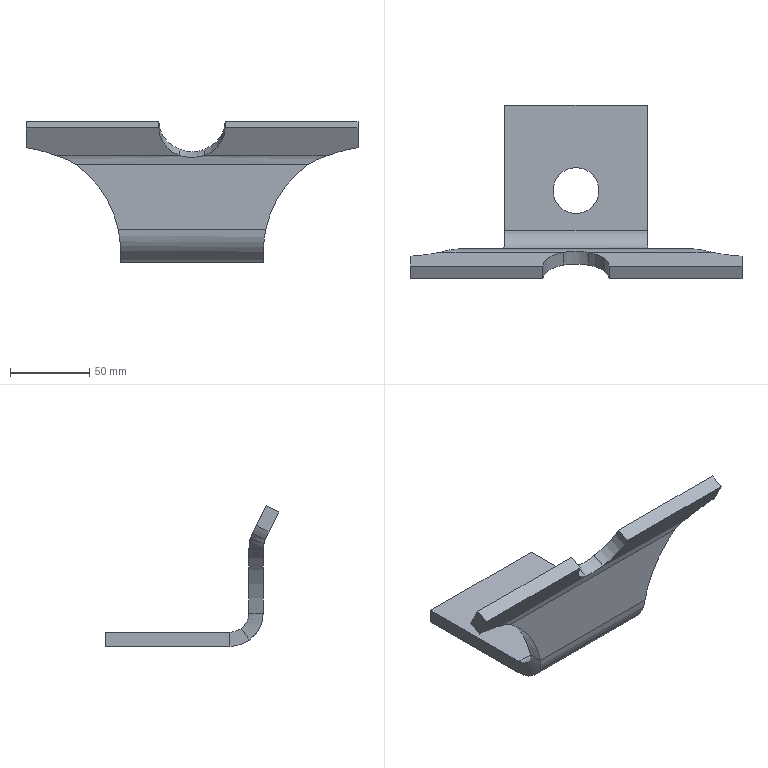Part | SolidWorks | features SM3dBend 2, FlatPattern 1, SMBaseFlange 1, SheetMetal 1, UnFold 1 | 1 solid | 34 faces | box 210 x 110.002 x 89.027 mm | volume 161533 mm3 | plane 17 | cylinder 12 | spline 5 | commonest cylinder face diameters 42 x4 140 x4 24 x2 29 x2
STEP:
#1=CARTESIAN_POINT('',(-14.5,118.35,9.));
#2=VERTEX_POINT('',#1);
#3=CARTESIAN_POINT('',(14.5,118.35,9.));
#4=VERTEX_POINT('',#3);
#5=CARTESIAN_POINT('',(0.,118.35,9.));
#6=DIRECTION('',(0.,0.,1.));
#7=DIRECTION('',(1.,0.,0.));
#8=AXIS2_PLACEMENT_3D('',#5,#6,#7);
#9=CIRCLE('',#8,14.5);
#10=EDGE_CURVE('',#2,#4,#9,.T.);
#11=ORIENTED_EDGE('',*,*,#10,.T.);
#12=CARTESIAN_POINT('',(14.5,118.35,0.));
#13=VERTEX_POINT('',#12);
#14=CARTESIAN_POINT('',(14.5,118.35,9.));
#15=DIRECTION('',(0.,0.,-1.));
#16=VECTOR('',#15,1000.);
#17=LINE('',#14,#16);
#18=EDGE_CURVE('',#4,#13,#17,.T.);
#19=ORIENTED_EDGE('',*,*,#18,.T.);
#20=CARTESIAN_POINT('',(-14.5,118.35,0.));
#21=VERTEX_POINT('',#20);
#22=CARTESIAN_POINT('',(0.,118.35,0.));
#23=DIRECTION('',(0.,0.,1.));
#24=DIRECTION('',(1.,0.,0.));
#25=AXIS2_PLACEMENT_3D('',#22,#23,#24);
#26=CIRCLE('',#25,14.5);
#27=EDGE_CURVE('',#21,#13,#26,.T.);
#28=ORIENTED_EDGE('',*,*,#27,.F.);
#29=CARTESIAN_POINT('',(-14.5,118.35,9.));
#30=DIRECTION('',(0.,0.,-1.));
#31=VECTOR('',#30,1000.);
#32=LINE('',#29,#31);
#33=EDGE_CURVE('',#2,#21,#32,.T.);
#34=ORIENTED_EDGE('',*,*,#33,.F.);
#35=EDGE_LOOP('',(#11,#19,#28,#34));
#36=FACE_OUTER_BOUND('',#35,.T.);
#37=CARTESIAN_POINT('',(0.,118.35,9.));
#38=DIRECTION('',(0.,0.,-1.));
#39=DIRECTION('',(-1.,0.,0.));
#40=AXIS2_PLACEMENT_3D('',#37,#38,#39);
#41=CYLINDRICAL_SURFACE('',#40,14.5);
#42=ADVANCED_FACE('',(#36),#41,.F.);
#43=CARTESIAN_POINT('',(-46.658,81.35,21.));
#44=VERTEX_POINT('',#43);
#45=CARTESIAN_POINT('',(-73.419,81.35,62.169));
#46=VERTEX_POINT('',#45);
#47=CARTESIAN_POINT('',(-115.,81.35,5.857));
#48=DIRECTION('',(0.,-1.,0.));
#49=DIRECTION('',(-1.,0.,0.));
#50=AXIS2_PLACEMENT_3D('',#47,#48,#49);
#51=CIRCLE('',#50,70.);
#52=EDGE_CURVE('',#44,#46,#51,.T.);
#53=ORIENTED_EDGE('',*,*,#52,.T.);
#54=CARTESIAN_POINT('',(73.419,81.35,62.169));
#55=VERTEX_POINT('',#54);
#56=CARTESIAN_POINT('',(115.,81.35,62.169));
#57=DIRECTION('',(1.,0.,0.));
#58=VECTOR('',#57,1000.);
#59=LINE('',#56,#58);
#60=EDGE_CURVE('',#46,#55,#59,.T.);
#61=ORIENTED_EDGE('',*,*,#60,.T.);
#62=CARTESIAN_POINT('',(46.658,81.35,21.));
#63=VERTEX_POINT('',#62);
#64=CARTESIAN_POINT('',(115.,81.35,5.857));
#65=DIRECTION('',(0.,-1.,0.));
#66=DIRECTION('',(1.,0.,0.));
#67=AXIS2_PLACEMENT_3D('',#64,#65,#66);
#68=CIRCLE('',#67,70.);
#69=EDGE_CURVE('',#55,#63,#68,.T.);
#70=ORIENTED_EDGE('',*,*,#69,.T.);
#71=CARTESIAN_POINT('',(115.,81.35,21.));
#72=DIRECTION('',(1.,0.,0.));
#73=VECTOR('',#72,1000.);
#74=LINE('',#71,#73);
#75=EDGE_CURVE('',#44,#63,#74,.T.);
#76=ORIENTED_EDGE('',*,*,#75,.F.);
#77=EDGE_LOOP('',(#53,#61,#70,#76));
#78=FACE_OUTER_BOUND('',#77,.T.);
#79=CARTESIAN_POINT('',(115.,81.35,5.857));
#80=DIRECTION('',(0.,1.,0.));
#81=DIRECTION('',(1.,0.,0.));
#82=AXIS2_PLACEMENT_3D('',#79,#80,#81);
#83=PLANE('',#82);
#84=ADVANCED_FACE('',(#78),#83,.T.);
#85=CARTESIAN_POINT('',(-73.419,72.35,62.169));
#86=VERTEX_POINT('',#85);
#87=CARTESIAN_POINT('',(-73.419,81.35,62.169));
#88=CARTESIAN_POINT('',(-73.419,72.35,62.169));
#89=B_SPLINE_CURVE_WITH_KNOTS('',1,(#87,#88),.UNSPECIFIED.,.F.,.F.,(2,2),(0.,1.),.UNSPECIFIED.);
#90=EDGE_CURVE('',#46,#86,#89,.T.);
#91=ORIENTED_EDGE('',*,*,#90,.F.);
#92=ORIENTED_EDGE('',*,*,#52,.F.);
#93=CARTESIAN_POINT('',(-46.658,72.35,21.));
#94=VERTEX_POINT('',#93);
#95=CARTESIAN_POINT('',(-46.658,81.35,21.));
#96=CARTESIAN_POINT('',(-46.658,78.35,21.));
#97=CARTESIAN_POINT('',(-46.658,75.35,21.));
#98=CARTESIAN_POINT('',(-46.658,72.35,21.));
#99=B_SPLINE_CURVE_WITH_KNOTS('',3,(#95,#96,#97,#98),.UNSPECIFIED.,.F.,.F.,(4,4),(0.,1.),.UNSPECIFIED.);
#100=EDGE_CURVE('',#44,#94,#99,.T.);
#101=ORIENTED_EDGE('',*,*,#100,.T.);
#102=CARTESIAN_POINT('',(-115.,72.35,5.857));
#103=DIRECTION('',(0.,-1.,0.));
#104=DIRECTION('',(-1.,0.,0.));
#105=AXIS2_PLACEMENT_3D('',#102,#103,#104);
#106=CIRCLE('',#105,70.);
#107=EDGE_CURVE('',#94,#86,#106,.T.);
#108=ORIENTED_EDGE('',*,*,#107,.T.);
#109=EDGE_LOOP('',(#91,#92,#101,#108));
#110=FACE_OUTER_BOUND('',#109,.T.);
#111=CARTESIAN_POINT('',(-115.,81.35,5.857));
#112=DIRECTION('',(0.,-1.,0.));
#113=DIRECTION('',(-1.,0.,0.));
#114=AXIS2_PLACEMENT_3D('',#111,#112,#113);
#115=CYLINDRICAL_SURFACE('',#114,70.);
#116=ADVANCED_FACE('',(#110),#115,.F.);
#117=CARTESIAN_POINT('',(73.419,72.35,62.169));
#118=VERTEX_POINT('',#117);
#119=CARTESIAN_POINT('',(73.419,72.35,62.169));
#120=CARTESIAN_POINT('',(73.419,81.35,62.169));
#121=B_SPLINE_CURVE_WITH_KNOTS('',1,(#119,#120),.UNSPECIFIED.,.F.,.F.,(2,2),(0.,1.),.UNSPECIFIED.);
#122=EDGE_CURVE('',#118,#55,#121,.T.);
#123=ORIENTED_EDGE('',*,*,#122,.F.);
#124=CARTESIAN_POINT('',(46.658,72.35,21.));
#125=VERTEX_POINT('',#124);
#126=CARTESIAN_POINT('',(115.,72.35,5.857));
#127=DIRECTION('',(0.,-1.,0.));
#128=DIRECTION('',(1.,0.,0.));
#129=AXIS2_PLACEMENT_3D('',#126,#127,#128);
#130=CIRCLE('',#129,70.);
#131=EDGE_CURVE('',#118,#125,#130,.T.);
#132=ORIENTED_EDGE('',*,*,#131,.T.);
#133=CARTESIAN_POINT('',(46.658,72.35,21.));
#134=CARTESIAN_POINT('',(46.658,75.35,21.));
#135=CARTESIAN_POINT('',(46.658,78.35,21.));
#136=CARTESIAN_POINT('',(46.658,81.35,21.));
#137=B_SPLINE_CURVE_WITH_KNOTS('',3,(#133,#134,#135,#136),.UNSPECIFIED.,.F.,.F.,(4,4),(0.,1.),.UNSPECIFIED.);
#138=EDGE_CURVE('',#125,#63,#137,.T.);
#139=ORIENTED_EDGE('',*,*,#138,.T.);
#140=ORIENTED_EDGE('',*,*,#69,.F.);
#141=EDGE_LOOP('',(#123,#132,#139,#140));
#142=FACE_OUTER_BOUND('',#141,.T.);
#143=CARTESIAN_POINT('',(115.,81.35,5.857));
#144=DIRECTION('',(0.,-1.,0.));
#145=DIRECTION('',(-1.,0.,0.));
#146=AXIS2_PLACEMENT_3D('',#143,#144,#145);
#147=CYLINDRICAL_SURFACE('',#146,70.);
#148=ADVANCED_FACE('',(#142),#147,.F.);
#149=CARTESIAN_POINT('',(115.,72.35,62.169));
#150=DIRECTION('',(1.,0.,0.));
#151=VECTOR('',#150,1000.);
#152=LINE('',#149,#151);
#153=EDGE_CURVE('',#86,#118,#152,.T.);
#154=ORIENTED_EDGE('',*,*,#153,.F.);
#155=ORIENTED_EDGE('',*,*,#107,.F.);
#156=CARTESIAN_POINT('',(115.,72.35,21.));
#157=DIRECTION('',(1.,0.,0.));
#158=VECTOR('',#157,1000.);
#159=LINE('',#156,#158);
#160=EDGE_CURVE('',#94,#125,#159,.T.);
#161=ORIENTED_EDGE('',*,*,#160,.T.);
#162=ORIENTED_EDGE('',*,*,#131,.F.);
#163=EDGE_LOOP('',(#154,#155,#161,#162));
#164=FACE_OUTER_BOUND('',#163,.T.);
#165=CARTESIAN_POINT('',(115.,72.35,5.857));
#166=DIRECTION('',(0.,1.,0.));
#167=DIRECTION('',(1.,0.,0.));
#168=AXIS2_PLACEMENT_3D('',#165,#166,#167);
#169=PLANE('',#168);
#170=ADVANCED_FACE('',(#164),#169,.F.);
#171=CARTESIAN_POINT('',(45.,172.35,0.));
#172=VERTEX_POINT('',#171);
#173=CARTESIAN_POINT('',(-45.,172.35,0.));
#174=VERTEX_POINT('',#173);
#175=CARTESIAN_POINT('',(45.,172.35,0.));
#176=DIRECTION('',(-1.,0.,0.));
#177=VECTOR('',#176,1000.);
#178=LINE('',#175,#177);
#179=EDGE_CURVE('',#172,#174,#178,.T.);
#180=ORIENTED_EDGE('',*,*,#179,.T.);
#181=CARTESIAN_POINT('',(-45.,172.35,9.));
#182=VERTEX_POINT('',#181);
#183=CARTESIAN_POINT('',(-45.,172.35,9.));
#184=DIRECTION('',(0.,0.,-1.));
#185=VECTOR('',#184,1000.);
#186=LINE('',#183,#185);
#187=EDGE_CURVE('',#182,#174,#186,.T.);
#188=ORIENTED_EDGE('',*,*,#187,.F.);
#189=CARTESIAN_POINT('',(45.,172.35,9.));
#190=VERTEX_POINT('',#189);
#191=CARTESIAN_POINT('',(45.,172.35,9.));
#192=DIRECTION('',(-1.,0.,0.));
#193=VECTOR('',#192,1000.);
#194=LINE('',#191,#193);
#195=EDGE_CURVE('',#190,#182,#194,.T.);
#196=ORIENTED_EDGE('',*,*,#195,.F.);
#197=CARTESIAN_POINT('',(45.,172.35,9.));
#198=DIRECTION('',(0.,0.,-1.));
#199=VECTOR('',#198,1000.);
#200=LINE('',#197,#199);
#201=EDGE_CURVE('',#190,#172,#200,.T.);
#202=ORIENTED_EDGE('',*,*,#201,.T.);
#203=EDGE_LOOP('',(#180,#188,#196,#202));
#204=FACE_OUTER_BOUND('',#203,.T.);
#205=CARTESIAN_POINT('',(45.,172.35,9.));
#206=DIRECTION('',(0.,-1.,0.));
#207=DIRECTION('',(0.,0.,-1.));
#208=AXIS2_PLACEMENT_3D('',#205,#206,#207);
#209=PLANE('',#208);
#210=ADVANCED_FACE('',(#204),#209,.F.);
#211=ORIENTED_EDGE('',*,*,#18,.F.);
#212=CARTESIAN_POINT('',(0.,118.35,9.));
#213=DIRECTION('',(0.,0.,1.));
#214=DIRECTION('',(1.,0.,0.));
#215=AXIS2_PLACEMENT_3D('',#212,#213,#214);
#216=CIRCLE('',#215,14.5);
#217=EDGE_CURVE('',#4,#2,#216,.T.);
#218=ORIENTED_EDGE('',*,*,#217,.T.);
#219=ORIENTED_EDGE('',*,*,#33,.T.);
#220=CARTESIAN_POINT('',(0.,118.35,0.));
#221=DIRECTION('',(0.,0.,1.));
#222=DIRECTION('',(1.,0.,0.));
#223=AXIS2_PLACEMENT_3D('',#220,#221,#222);
#224=CIRCLE('',#223,14.5);
#225=EDGE_CURVE('',#13,#21,#224,.T.);
#226=ORIENTED_EDGE('',*,*,#225,.F.);
#227=EDGE_LOOP('',(#211,#218,#219,#226));
#228=FACE_OUTER_BOUND('',#227,.T.);
#229=CARTESIAN_POINT('',(0.,118.35,9.));
#230=DIRECTION('',(0.,0.,-1.));
#231=DIRECTION('',(-1.,0.,0.));
#232=AXIS2_PLACEMENT_3D('',#229,#230,#231);
#233=CYLINDRICAL_SURFACE('',#232,14.5);
#234=ADVANCED_FACE('',(#228),#233,.F.);
#235=ORIENTED_EDGE('',*,*,#10,.F.);
#236=ORIENTED_EDGE('',*,*,#217,.F.);
#237=EDGE_LOOP('',(#235,#236));
#238=FACE_BOUND('',#237,.T.);
#239=CARTESIAN_POINT('',(-45.,93.35,9.));
#240=VERTEX_POINT('',#239);
#241=CARTESIAN_POINT('',(-45.,83.282,9.));
#242=DIRECTION('',(0.,-1.,0.));
#243=VECTOR('',#242,1000.);
#244=LINE('',#241,#243);
#245=EDGE_CURVE('',#182,#240,#244,.T.);
#246=ORIENTED_EDGE('',*,*,#245,.T.);
#247=CARTESIAN_POINT('',(45.,93.35,9.));
#248=VERTEX_POINT('',#247);
#249=CARTESIAN_POINT('',(115.,93.35,9.));
#250=DIRECTION('',(1.,0.,0.));
#251=VECTOR('',#250,1000.);
#252=LINE('',#249,#251);
#253=EDGE_CURVE('',#240,#248,#252,.T.);
#254=ORIENTED_EDGE('',*,*,#253,.T.);
#255=CARTESIAN_POINT('',(45.,83.282,9.));
#256=DIRECTION('',(0.,1.,0.));
#257=VECTOR('',#256,1000.);
#258=LINE('',#255,#257);
#259=EDGE_CURVE('',#248,#190,#258,.T.);
#260=ORIENTED_EDGE('',*,*,#259,.T.);
#261=ORIENTED_EDGE('',*,*,#195,.T.);
#262=EDGE_LOOP('',(#246,#254,#260,#261));
#263=FACE_OUTER_BOUND('',#262,.T.);
#264=CARTESIAN_POINT('',(115.,83.282,9.));
#265=DIRECTION('',(0.,0.,1.));
#266=DIRECTION('',(1.,0.,0.));
#267=AXIS2_PLACEMENT_3D('',#264,#265,#266);
#268=PLANE('',#267);
#269=ADVANCED_FACE('',(#238,#263),#268,.T.);
#270=CARTESIAN_POINT('',(45.,93.35,0.));
#271=VERTEX_POINT('',#270);
#272=CARTESIAN_POINT('',(45.,93.35,9.));
#273=DIRECTION('',(0.,0.,1.));
#274=VECTOR('',#273,1000.);
#275=LINE('',#272,#274);
#276=EDGE_CURVE('',#271,#248,#275,.T.);
#277=ORIENTED_EDGE('',*,*,#276,.F.);
#278=CARTESIAN_POINT('',(45.,83.282,0.));
#279=DIRECTION('',(0.,1.,0.));
#280=VECTOR('',#279,1000.);
#281=LINE('',#278,#280);
#282=EDGE_CURVE('',#271,#172,#281,.T.);
#283=ORIENTED_EDGE('',*,*,#282,.T.);
#284=ORIENTED_EDGE('',*,*,#201,.F.);
#285=ORIENTED_EDGE('',*,*,#259,.F.);
#286=EDGE_LOOP('',(#277,#283,#284,#285));
#287=FACE_OUTER_BOUND('',#286,.T.);
#288=CARTESIAN_POINT('',(45.,83.282,9.));
#289=DIRECTION('',(-1.,0.,0.));
#290=DIRECTION('',(0.,0.,1.));
#291=AXIS2_PLACEMENT_3D('',#288,#289,#290);
#292=PLANE('',#291);
#293=ADVANCED_FACE('',(#287),#292,.F.);
#294=CARTESIAN_POINT('',(-45.,93.35,0.));
#295=VERTEX_POINT('',#294);
#296=CARTESIAN_POINT('',(115.,93.35,0.));
#297=DIRECTION('',(1.,0.,0.));
#298=VECTOR('',#297,1000.);
#299=LINE('',#296,#298);
#300=EDGE_CURVE('',#295,#271,#299,.T.);
#301=ORIENTED_EDGE('',*,*,#300,.F.);
#302=CARTESIAN_POINT('',(-45.,83.282,0.));
#303=DIRECTION('',(0.,-1.,0.));
#304=VECTOR('',#303,1000.);
#305=LINE('',#302,#304);
#306=EDGE_CURVE('',#174,#295,#305,.T.);
#307=ORIENTED_EDGE('',*,*,#306,.F.);
#308=ORIENTED_EDGE('',*,*,#179,.F.);
#309=ORIENTED_EDGE('',*,*,#282,.F.);
#310=EDGE_LOOP('',(#301,#307,#308,#309));
#311=FACE_OUTER_BOUND('',#310,.T.);
#312=ORIENTED_EDGE('',*,*,#27,.T.);
#313=ORIENTED_EDGE('',*,*,#225,.T.);
#314=EDGE_LOOP('',(#312,#313));
#315=FACE_BOUND('',#314,.T.);
#316=CARTESIAN_POINT('',(115.,83.282,0.));
#317=DIRECTION('',(0.,0.,1.));
#318=DIRECTION('',(1.,0.,0.));
#319=AXIS2_PLACEMENT_3D('',#316,#317,#318);
#320=PLANE('',#319);
#321=ADVANCED_FACE('',(#311,#315),#320,.F.);
#322=CARTESIAN_POINT('',(-45.,93.35,9.));
#323=DIRECTION('',(0.,0.,-1.));
#324=VECTOR('',#323,1000.);
#325=LINE('',#322,#324);
#326=EDGE_CURVE('',#240,#295,#325,.T.);
#327=ORIENTED_EDGE('',*,*,#326,.F.);
#328=ORIENTED_EDGE('',*,*,#245,.F.);
#329=ORIENTED_EDGE('',*,*,#187,.T.);
#330=ORIENTED_EDGE('',*,*,#306,.T.);
#331=EDGE_LOOP('',(#327,#328,#329,#330));
#332=FACE_OUTER_BOUND('',#331,.T.);
#333=CARTESIAN_POINT('',(-45.,83.282,9.));
#334=DIRECTION('',(1.,0.,0.));
#335=DIRECTION('',(0.,0.,-1.));
#336=AXIS2_PLACEMENT_3D('',#333,#334,#335);
#337=PLANE('',#336);
#338=ADVANCED_FACE('',(#332),#337,.F.);
#339=CARTESIAN_POINT('',(-45.,81.024,3.998));
#340=VERTEX_POINT('',#339);
#341=CARTESIAN_POINT('',(-45.,86.307,11.285));
#342=VERTEX_POINT('',#341);
#343=CARTESIAN_POINT('',(-45.,81.024,3.998));
#344=CARTESIAN_POINT('',(-45.,82.785,6.427));
#345=CARTESIAN_POINT('',(-45.,84.546,8.856));
#346=CARTESIAN_POINT('',(-45.,86.307,11.285));
#347=B_SPLINE_CURVE_WITH_KNOTS('',3,(#343,#344,#345,#346),.UNSPECIFIED.,.F.,.F.,(4,4),(0.,1.),.UNSPECIFIED.);
#348=EDGE_CURVE('',#340,#342,#347,.T.);
#349=ORIENTED_EDGE('',*,*,#348,.F.);
#350=CARTESIAN_POINT('',(-45.,81.024,3.998));
#351=CARTESIAN_POINT('',(-45.037,79.286,5.258));
#352=CARTESIAN_POINT('',(-45.09,77.943,6.633));
#353=CARTESIAN_POINT('',(-45.193,76.386,8.593));
#354=CARTESIAN_POINT('',(-45.231,75.943,9.231));
#355=CARTESIAN_POINT('',(-45.294,75.372,10.141));
#356=CARTESIAN_POINT('',(-45.316,75.197,10.436));
#357=CARTESIAN_POINT('',(-45.362,74.876,11.009));
#358=CARTESIAN_POINT('',(-45.385,74.733,11.278));
#359=CARTESIAN_POINT('',(-45.513,74.041,12.652));
#360=CARTESIAN_POINT('',(-45.669,73.49,13.982));
#361=CARTESIAN_POINT('',(-46.084,72.644,17.137));
#362=CARTESIAN_POINT('',(-46.344,72.35,18.962));
#363=CARTESIAN_POINT('',(-46.658,72.35,21.));
#364=B_SPLINE_CURVE_WITH_KNOTS('',3,(#350,#351,#352,#353,#354,#355,#356,#357,#358,#359,#360,#361,#362,#363),.UNSPECIFIED.,.F.,.F.,(4,2,2,2,2,2,4),(0.,0.25,0.375,0.4375,0.5,0.75,1.),.UNSPECIFIED.);
#365=EDGE_CURVE('',#340,#94,#364,.T.);
#366=ORIENTED_EDGE('',*,*,#365,.T.);
#367=ORIENTED_EDGE('',*,*,#100,.F.);
#368=CARTESIAN_POINT('',(-45.,86.307,11.285));
#369=CARTESIAN_POINT('',(-45.037,85.315,12.003));
#370=CARTESIAN_POINT('',(-45.09,84.546,12.79));
#371=CARTESIAN_POINT('',(-45.193,83.656,13.91));
#372=CARTESIAN_POINT('',(-45.231,83.403,14.275));
#373=CARTESIAN_POINT('',(-45.294,83.077,14.795));
#374=CARTESIAN_POINT('',(-45.316,82.977,14.964));
#375=CARTESIAN_POINT('',(-45.35,82.839,15.209));
#376=CARTESIAN_POINT('',(-45.368,82.773,15.33));
#377=CARTESIAN_POINT('',(-45.386,82.712,15.447));
#378=CARTESIAN_POINT('',(-45.398,82.672,15.525));
#379=CARTESIAN_POINT('',(-45.404,82.653,15.562));
#380=CARTESIAN_POINT('',(-45.513,82.317,16.23));
#381=CARTESIAN_POINT('',(-45.669,82.002,16.99));
#382=CARTESIAN_POINT('',(-46.084,81.518,18.792));
#383=CARTESIAN_POINT('',(-46.345,81.35,19.837));
#384=CARTESIAN_POINT('',(-46.658,81.35,21.));
#385=B_SPLINE_CURVE_WITH_KNOTS('',3,(#368,#369,#370,#371,#372,#373,#374,#375,#376,#377,#378,#379,#380,#381,#382,#383,#384),.UNSPECIFIED.,.F.,.F.,(4,2,2,2,1,2,2,2,4),(0.,0.25,0.375,0.4375,0.4688,0.4844,0.5,0.75,1.),.UNSPECIFIED.);
#386=EDGE_CURVE('',#342,#44,#385,.T.);
#387=ORIENTED_EDGE('',*,*,#386,.F.);
#388=EDGE_LOOP('',(#349,#366,#367,#387));
#389=FACE_OUTER_BOUND('',#388,.T.);
#390=CARTESIAN_POINT('',(-45.,81.024,3.998));
#391=CARTESIAN_POINT('',(-45.037,79.286,5.258));
#392=CARTESIAN_POINT('',(-45.09,77.943,6.633));
#393=CARTESIAN_POINT('',(-45.193,76.386,8.593));
#394=CARTESIAN_POINT('',(-45.231,75.943,9.231));
#395=CARTESIAN_POINT('',(-45.294,75.372,10.141));
#396=CARTESIAN_POINT('',(-45.316,75.197,10.436));
#397=CARTESIAN_POINT('',(-45.362,74.876,11.009));
#398=CARTESIAN_POINT('',(-45.385,74.733,11.278));
#399=CARTESIAN_POINT('',(-45.513,74.041,12.652));
#400=CARTESIAN_POINT('',(-45.669,73.49,13.982));
#401=CARTESIAN_POINT('',(-46.084,72.644,17.137));
#402=CARTESIAN_POINT('',(-46.344,72.35,18.962));
#403=CARTESIAN_POINT('',(-46.658,72.35,21.));
#404=CARTESIAN_POINT('',(-45.,86.307,11.285));
#405=CARTESIAN_POINT('',(-45.037,85.314,12.004));
#406=CARTESIAN_POINT('',(-45.09,84.546,12.79));
#407=CARTESIAN_POINT('',(-45.193,83.656,13.91));
#408=CARTESIAN_POINT('',(-45.231,83.403,14.275));
#409=CARTESIAN_POINT('',(-45.294,83.077,14.795));
#410=CARTESIAN_POINT('',(-45.316,82.977,14.964));
#411=CARTESIAN_POINT('',(-45.362,82.793,15.291));
#412=CARTESIAN_POINT('',(-45.385,82.712,15.445));
#413=CARTESIAN_POINT('',(-45.513,82.317,16.23));
#414=CARTESIAN_POINT('',(-45.669,82.002,16.99));
#415=CARTESIAN_POINT('',(-46.084,81.518,18.792));
#416=CARTESIAN_POINT('',(-46.344,81.35,19.835));
#417=CARTESIAN_POINT('',(-46.658,81.35,21.));
#418=B_SPLINE_SURFACE_WITH_KNOTS('',1,3,((#390,#391,#392,#393,#394,#395,#396,#397,#398,#399,#400,#401,#402,#403),(#404,#405,#406,#407,#408,#409,#410,#411,#412,#413,#414,#415,#416,#417)),.UNSPECIFIED.,.F.,.F.,.F.,(2,2),(4,2,2,2,2,2,4),(0.,1.),(0.,0.25,0.375,0.4375,0.5,0.75,1.),.UNSPECIFIED.);
#419=ADVANCED_FACE('',(#389),#418,.F.);
#420=ORIENTED_EDGE('',*,*,#138,.F.);
#421=CARTESIAN_POINT('',(45.,81.024,3.998));
#422=VERTEX_POINT('',#421);
#423=CARTESIAN_POINT('',(46.658,72.35,21.));
#424=CARTESIAN_POINT('',(46.342,72.35,18.923));
#425=CARTESIAN_POINT('',(46.081,72.655,17.08));
#426=CARTESIAN_POINT('',(45.769,73.296,14.715));
#427=CARTESIAN_POINT('',(45.679,73.541,13.993));
#428=CARTESIAN_POINT('',(45.563,73.928,13.006));
#429=CARTESIAN_POINT('',(45.528,74.06,12.693));
#430=CARTESIAN_POINT('',(45.464,74.327,12.099));
#431=CARTESIAN_POINT('',(45.436,74.458,11.826));
#432=CARTESIAN_POINT('',(45.306,75.15,10.452));
#433=CARTESIAN_POINT('',(45.22,75.899,9.2));
#434=CARTESIAN_POINT('',(45.083,77.981,6.592));
#435=CARTESIAN_POINT('',(45.033,79.316,5.236));
#436=CARTESIAN_POINT('',(45.,81.024,3.998));
#437=B_SPLINE_CURVE_WITH_KNOTS('',3,(#423,#424,#425,#426,#427,#428,#429,#430,#431,#432,#433,#434,#435,#436),.UNSPECIFIED.,.F.,.F.,(4,2,2,2,2,2,4),(0.,0.25,0.375,0.4375,0.5,0.75,1.),.UNSPECIFIED.);
#438=EDGE_CURVE('',#125,#422,#437,.T.);
#439=ORIENTED_EDGE('',*,*,#438,.T.);
#440=CARTESIAN_POINT('',(45.,86.307,11.285));
#441=VERTEX_POINT('',#440);
#442=CARTESIAN_POINT('',(45.,81.024,3.998));
#443=CARTESIAN_POINT('',(45.,86.307,11.285));
#444=B_SPLINE_CURVE_WITH_KNOTS('',1,(#442,#443),.UNSPECIFIED.,.F.,.F.,(2,2),(0.,1.),.UNSPECIFIED.);
#445=EDGE_CURVE('',#422,#441,#444,.T.);
#446=ORIENTED_EDGE('',*,*,#445,.T.);
#447=CARTESIAN_POINT('',(46.658,81.35,21.));
#448=CARTESIAN_POINT('',(46.343,81.35,19.815));
#449=CARTESIAN_POINT('',(46.081,81.524,18.76));
#450=CARTESIAN_POINT('',(45.769,81.89,17.409));
#451=CARTESIAN_POINT('',(45.679,82.031,16.996));
#452=CARTESIAN_POINT('',(45.563,82.252,16.432));
#453=CARTESIAN_POINT('',(45.528,82.327,16.253));
#454=CARTESIAN_POINT('',(45.48,82.442,15.998));
#455=CARTESIAN_POINT('',(45.457,82.499,15.874));
#456=CARTESIAN_POINT('',(45.436,82.557,15.755));
#457=CARTESIAN_POINT('',(45.423,82.595,15.677));
#458=CARTESIAN_POINT('',(45.417,82.614,15.64));
#459=CARTESIAN_POINT('',(45.306,82.95,14.972));
#460=CARTESIAN_POINT('',(45.22,83.378,14.257));
#461=CARTESIAN_POINT('',(45.083,84.568,12.767));
#462=CARTESIAN_POINT('',(45.033,85.332,11.991));
#463=CARTESIAN_POINT('',(45.,86.307,11.285));
#464=B_SPLINE_CURVE_WITH_KNOTS('',3,(#447,#448,#449,#450,#451,#452,#453,#454,#455,#456,#457,#458,#459,#460,#461,#462,#463),.UNSPECIFIED.,.F.,.F.,(4,2,2,2,1,2,2,2,4),(0.,0.25,0.375,0.4375,0.4688,0.4844,0.5,0.75,1.),.UNSPECIFIED.);
#465=EDGE_CURVE('',#63,#441,#464,.T.);
#466=ORIENTED_EDGE('',*,*,#465,.F.);
#467=EDGE_LOOP('',(#420,#439,#446,#466));
#468=FACE_OUTER_BOUND('',#467,.T.);
#469=CARTESIAN_POINT('',(46.658,72.35,21.));
#470=CARTESIAN_POINT('',(46.342,72.35,18.923));
#471=CARTESIAN_POINT('',(46.081,72.655,17.08));
#472=CARTESIAN_POINT('',(45.769,73.296,14.715));
#473=CARTESIAN_POINT('',(45.679,73.541,13.993));
#474=CARTESIAN_POINT('',(45.563,73.928,13.006));
#475=CARTESIAN_POINT('',(45.528,74.06,12.693));
#476=CARTESIAN_POINT('',(45.464,74.327,12.099));
#477=CARTESIAN_POINT('',(45.436,74.458,11.826));
#478=CARTESIAN_POINT('',(45.306,75.15,10.452));
#479=CARTESIAN_POINT('',(45.22,75.899,9.2));
#480=CARTESIAN_POINT('',(45.083,77.981,6.592));
#481=CARTESIAN_POINT('',(45.033,79.316,5.236));
#482=CARTESIAN_POINT('',(45.,81.024,3.998));
#483=CARTESIAN_POINT('',(46.658,81.35,21.));
#484=CARTESIAN_POINT('',(46.342,81.35,19.813));
#485=CARTESIAN_POINT('',(46.081,81.524,18.76));
#486=CARTESIAN_POINT('',(45.769,81.89,17.409));
#487=CARTESIAN_POINT('',(45.679,82.031,16.996));
#488=CARTESIAN_POINT('',(45.563,82.252,16.432));
#489=CARTESIAN_POINT('',(45.528,82.327,16.253));
#490=CARTESIAN_POINT('',(45.464,82.48,15.914));
#491=CARTESIAN_POINT('',(45.436,82.554,15.757));
#492=CARTESIAN_POINT('',(45.306,82.95,14.972));
#493=CARTESIAN_POINT('',(45.22,83.378,14.257));
#494=CARTESIAN_POINT('',(45.083,84.568,12.767));
#495=CARTESIAN_POINT('',(45.033,85.331,11.992));
#496=CARTESIAN_POINT('',(45.,86.307,11.285));
#497=B_SPLINE_SURFACE_WITH_KNOTS('',1,3,((#469,#470,#471,#472,#473,#474,#475,#476,#477,#478,#479,#480,#481,#482),(#483,#484,#485,#486,#487,#488,#489,#490,#491,#492,#493,#494,#495,#496)),.UNSPECIFIED.,.F.,.F.,.F.,(2,2),(4,2,2,2,2,2,4),(0.,1.),(0.,0.25,0.375,0.4375,0.5,0.75,1.),.UNSPECIFIED.);
#498=ADVANCED_FACE('',(#468),#497,.F.);
#499=ORIENTED_EDGE('',*,*,#445,.F.);
#500=CARTESIAN_POINT('',(45.,93.35,21.));
#501=DIRECTION('',(1.,0.,0.));
#502=DIRECTION('',(0.,1.,0.));
#503=AXIS2_PLACEMENT_3D('',#500,#501,#502);
#504=CIRCLE('',#503,21.);
#505=EDGE_CURVE('',#422,#271,#504,.T.);
#506=ORIENTED_EDGE('',*,*,#505,.T.);
#507=ORIENTED_EDGE('',*,*,#276,.T.);
#508=CARTESIAN_POINT('',(45.,93.35,21.));
#509=DIRECTION('',(1.,0.,0.));
#510=DIRECTION('',(0.,0.,-1.));
#511=AXIS2_PLACEMENT_3D('',#508,#509,#510);
#512=CIRCLE('',#511,12.);
#513=EDGE_CURVE('',#441,#248,#512,.T.);
#514=ORIENTED_EDGE('',*,*,#513,.F.);
#515=EDGE_LOOP('',(#499,#506,#507,#514));
#516=FACE_OUTER_BOUND('',#515,.T.);
#517=CARTESIAN_POINT('',(45.,93.35,21.));
#518=DIRECTION('',(-1.,0.,0.));
#519=DIRECTION('',(0.,0.,1.));
#520=AXIS2_PLACEMENT_3D('',#517,#518,#519);
#521=PLANE('',#520);
#522=ADVANCED_FACE('',(#516),#521,.F.);
#523=CARTESIAN_POINT('',(-45.,93.35,21.));
#524=DIRECTION('',(-1.,0.,0.));
#525=DIRECTION('',(0.,1.,0.));
#526=AXIS2_PLACEMENT_3D('',#523,#524,#525);
#527=CIRCLE('',#526,21.);
#528=EDGE_CURVE('',#295,#340,#527,.T.);
#529=ORIENTED_EDGE('',*,*,#528,.T.);
#530=ORIENTED_EDGE('',*,*,#348,.T.);
#531=CARTESIAN_POINT('',(-45.,93.35,21.));
#532=DIRECTION('',(-1.,0.,0.));
#533=DIRECTION('',(0.,0.,1.));
#534=AXIS2_PLACEMENT_3D('',#531,#532,#533);
#535=CIRCLE('',#534,12.);
#536=EDGE_CURVE('',#240,#342,#535,.T.);
#537=ORIENTED_EDGE('',*,*,#536,.F.);
#538=ORIENTED_EDGE('',*,*,#326,.T.);
#539=EDGE_LOOP('',(#529,#530,#537,#538));
#540=FACE_OUTER_BOUND('',#539,.T.);
#541=CARTESIAN_POINT('',(-45.,93.35,21.));
#542=DIRECTION('',(1.,0.,0.));
#543=DIRECTION('',(0.,0.,-1.));
#544=AXIS2_PLACEMENT_3D('',#541,#542,#543);
#545=PLANE('',#544);
#546=ADVANCED_FACE('',(#540),#545,.F.);
#547=ORIENTED_EDGE('',*,*,#253,.F.);
#548=ORIENTED_EDGE('',*,*,#536,.T.);
#549=ORIENTED_EDGE('',*,*,#386,.T.);
#550=ORIENTED_EDGE('',*,*,#75,.T.);
#551=ORIENTED_EDGE('',*,*,#465,.T.);
#552=ORIENTED_EDGE('',*,*,#513,.T.);
#553=EDGE_LOOP('',(#547,#548,#549,#550,#551,#552));
#554=FACE_OUTER_BOUND('',#553,.T.);
#555=CARTESIAN_POINT('',(-97.079,93.35,21.));
#556=DIRECTION('',(1.,0.,0.));
#557=DIRECTION('',(0.,1.,0.));
#558=AXIS2_PLACEMENT_3D('',#555,#556,#557);
#559=CYLINDRICAL_SURFACE('',#558,12.);
#560=ADVANCED_FACE('',(#554),#559,.F.);
#561=ORIENTED_EDGE('',*,*,#300,.T.);
#562=ORIENTED_EDGE('',*,*,#505,.F.);
#563=ORIENTED_EDGE('',*,*,#438,.F.);
#564=ORIENTED_EDGE('',*,*,#160,.F.);
#565=ORIENTED_EDGE('',*,*,#365,.F.);
#566=ORIENTED_EDGE('',*,*,#528,.F.);
#567=EDGE_LOOP('',(#561,#562,#563,#564,#565,#566));
#568=FACE_OUTER_BOUND('',#567,.T.);
#569=CARTESIAN_POINT('',(-97.079,93.35,21.));
#570=DIRECTION('',(1.,0.,0.));
#571=DIRECTION('',(0.,1.,0.));
#572=AXIS2_PLACEMENT_3D('',#569,#570,#571);
#573=CYLINDRICAL_SURFACE('',#572,21.);
#574=ADVANCED_FACE('',(#568),#573,.T.);
#575=ORIENTED_EDGE('',*,*,#90,.T.);
#576=CARTESIAN_POINT('',(-86.098,71.083,67.536));
#577=VERTEX_POINT('',#576);
#578=CARTESIAN_POINT('',(-73.419,72.35,62.169));
#579=CARTESIAN_POINT('',(-74.696,72.35,62.841));
#580=CARTESIAN_POINT('',(-75.839,72.294,63.426));
#581=CARTESIAN_POINT('',(-77.352,72.185,64.167));
#582=CARTESIAN_POINT('',(-77.822,72.144,64.392));
#583=CARTESIAN_POINT('',(-78.478,72.081,64.695));
#584=CARTESIAN_POINT('',(-78.688,72.06,64.791));
#585=CARTESIAN_POINT('',(-78.991,72.029,64.926));
#586=CARTESIAN_POINT('',(-79.09,72.019,64.97));
#587=CARTESIAN_POINT('',(-79.235,72.003,65.033));
#588=CARTESIAN_POINT('',(-79.282,71.998,65.054));
#589=CARTESIAN_POINT('',(-79.377,71.988,65.095));
#590=CARTESIAN_POINT('',(-79.419,71.983,65.113));
#591=CARTESIAN_POINT('',(-81.108,71.799,65.836));
#592=CARTESIAN_POINT('',(-83.317,71.525,66.652));
#593=CARTESIAN_POINT('',(-86.098,71.083,67.536));
#594=B_SPLINE_CURVE_WITH_KNOTS('',3,(#578,#579,#580,#581,#582,#583,#584,#585,#586,#587,#588,#589,#590,#591,#592,#593),.UNSPECIFIED.,.F.,.F.,(4,2,2,2,2,2,2,4),(0.,0.25,0.375,0.4375,0.4688,0.4844,0.5,1.),.UNSPECIFIED.);
#595=EDGE_CURVE('',#86,#577,#594,.T.);
#596=ORIENTED_EDGE('',*,*,#595,.T.);
#597=CARTESIAN_POINT('',(-86.098,79.132,71.562));
#598=VERTEX_POINT('',#597);
#599=CARTESIAN_POINT('',(-86.098,79.132,71.562));
#600=CARTESIAN_POINT('',(-86.098,76.449,70.22));
#601=CARTESIAN_POINT('',(-86.098,73.766,68.878));
#602=CARTESIAN_POINT('',(-86.098,71.083,67.536));
#603=B_SPLINE_CURVE_WITH_KNOTS('',3,(#599,#600,#601,#602),.UNSPECIFIED.,.F.,.F.,(4,4),(0.,1.),.UNSPECIFIED.);
#604=EDGE_CURVE('',#598,#577,#603,.T.);
#605=ORIENTED_EDGE('',*,*,#604,.F.);
#606=CARTESIAN_POINT('',(-73.419,81.35,62.169));
#607=CARTESIAN_POINT('',(-74.696,81.35,63.345));
#608=CARTESIAN_POINT('',(-75.839,81.253,64.368));
#609=CARTESIAN_POINT('',(-77.352,81.061,65.666));
#610=CARTESIAN_POINT('',(-77.822,80.99,66.059));
#611=CARTESIAN_POINT('',(-78.478,80.88,66.59));
#612=CARTESIAN_POINT('',(-78.688,80.843,66.758));
#613=CARTESIAN_POINT('',(-78.991,80.788,66.994));
#614=CARTESIAN_POINT('',(-79.139,80.761,67.109));
#615=CARTESIAN_POINT('',(-79.306,80.729,67.237));
#616=CARTESIAN_POINT('',(-79.389,80.714,67.299));
#617=CARTESIAN_POINT('',(-79.424,80.707,67.325));
#618=CARTESIAN_POINT('',(-79.447,80.703,67.343));
#619=CARTESIAN_POINT('',(-79.457,80.701,67.35));
#620=CARTESIAN_POINT('',(-80.289,80.542,67.974));
#621=CARTESIAN_POINT('',(-81.251,80.343,68.636));
#622=CARTESIAN_POINT('',(-83.46,79.832,70.044));
#623=CARTESIAN_POINT('',(-84.707,79.519,70.789));
#624=CARTESIAN_POINT('',(-86.098,79.132,71.562));
#625=B_SPLINE_CURVE_WITH_KNOTS('',3,(#606,#607,#608,#609,#610,#611,#612,#613,#614,#615,#616,#617,#618,#619,#620,#621,#622,#623,#624),.UNSPECIFIED.,.F.,.F.,(4,2,2,2,1,1,1,2,2,2,4),(0.,0.25,0.375,0.4375,0.4687,0.4844,0.4922,0.4961,0.5,0.75,1.),.UNSPECIFIED.);
#626=EDGE_CURVE('',#46,#598,#625,.T.);
#627=ORIENTED_EDGE('',*,*,#626,.F.);
#628=EDGE_LOOP('',(#575,#596,#605,#627));
#629=FACE_OUTER_BOUND('',#628,.T.);
#630=CARTESIAN_POINT('',(-73.419,81.35,62.169));
#631=CARTESIAN_POINT('',(-74.696,81.35,63.345));
#632=CARTESIAN_POINT('',(-75.839,81.253,64.368));
#633=CARTESIAN_POINT('',(-77.352,81.061,65.666));
#634=CARTESIAN_POINT('',(-77.822,80.99,66.059));
#635=CARTESIAN_POINT('',(-78.478,80.88,66.59));
#636=CARTESIAN_POINT('',(-78.688,80.843,66.758));
#637=CARTESIAN_POINT('',(-78.991,80.788,66.994));
#638=CARTESIAN_POINT('',(-79.09,80.77,67.071));
#639=CARTESIAN_POINT('',(-79.235,80.743,67.182));
#640=CARTESIAN_POINT('',(-79.282,80.734,67.218));
#641=CARTESIAN_POINT('',(-79.377,80.716,67.29));
#642=CARTESIAN_POINT('',(-79.419,80.708,67.322));
#643=CARTESIAN_POINT('',(-81.108,80.385,68.587));
#644=CARTESIAN_POINT('',(-83.316,79.906,70.015));
#645=CARTESIAN_POINT('',(-86.098,79.132,71.562));
#646=CARTESIAN_POINT('',(-73.419,72.35,62.169));
#647=CARTESIAN_POINT('',(-74.696,72.35,62.841));
#648=CARTESIAN_POINT('',(-75.839,72.294,63.426));
#649=CARTESIAN_POINT('',(-77.352,72.185,64.167));
#650=CARTESIAN_POINT('',(-77.822,72.144,64.392));
#651=CARTESIAN_POINT('',(-78.478,72.081,64.695));
#652=CARTESIAN_POINT('',(-78.688,72.06,64.791));
#653=CARTESIAN_POINT('',(-78.991,72.029,64.926));
#654=CARTESIAN_POINT('',(-79.09,72.019,64.97));
#655=CARTESIAN_POINT('',(-79.235,72.003,65.033));
#656=CARTESIAN_POINT('',(-79.282,71.998,65.054));
#657=CARTESIAN_POINT('',(-79.377,71.988,65.095));
#658=CARTESIAN_POINT('',(-79.419,71.983,65.113));
#659=CARTESIAN_POINT('',(-81.108,71.799,65.836));
#660=CARTESIAN_POINT('',(-83.317,71.525,66.652));
#661=CARTESIAN_POINT('',(-86.098,71.083,67.536));
#662=B_SPLINE_SURFACE_WITH_KNOTS('',1,3,((#630,#631,#632,#633,#634,#635,#636,#637,#638,#639,#640,#641,#642,#643,#644,#645),(#646,#647,#648,#649,#650,#651,#652,#653,#654,#655,#656,#657,#658,#659,#660,#661)),.UNSPECIFIED.,.F.,.F.,.F.,(2,2),(4,2,2,2,2,2,2,4),(0.,1.),(0.,0.25,0.375,0.4375,0.4688,0.4844,0.5,1.),.UNSPECIFIED.);
#663=ADVANCED_FACE('',(#629),#662,.T.);
#664=CARTESIAN_POINT('',(-7.726,71.083,67.536));
#665=VERTEX_POINT('',#664);
#666=CARTESIAN_POINT('',(-7.726,79.132,71.562));
#667=VERTEX_POINT('',#666);
#668=CARTESIAN_POINT('',(-7.726,71.083,67.536));
#669=CARTESIAN_POINT('',(-7.726,73.766,68.878));
#670=CARTESIAN_POINT('',(-7.726,76.449,70.22));
#671=CARTESIAN_POINT('',(-7.726,79.132,71.562));
#672=B_SPLINE_CURVE_WITH_KNOTS('',3,(#668,#669,#670,#671),.UNSPECIFIED.,.F.,.F.,(4,4),(0.,1.),.UNSPECIFIED.);
#673=EDGE_CURVE('',#665,#667,#672,.T.);
#674=ORIENTED_EDGE('',*,*,#673,.F.);
#675=CARTESIAN_POINT('',(7.726,71.083,67.536));
#676=VERTEX_POINT('',#675);
#677=CARTESIAN_POINT('',(-7.726,71.083,67.536));
#678=CARTESIAN_POINT('',(-6.939,71.175,67.351));
#679=CARTESIAN_POINT('',(-6.234,71.247,67.196));
#680=CARTESIAN_POINT('',(-5.297,71.331,67.008));
#681=CARTESIAN_POINT('',(-5.006,71.355,66.954));
#682=CARTESIAN_POINT('',(-4.599,71.385,66.884));
#683=CARTESIAN_POINT('',(-4.468,71.394,66.862));
#684=CARTESIAN_POINT('',(-4.28,71.406,66.833));
#685=CARTESIAN_POINT('',(-4.218,71.41,66.824));
#686=CARTESIAN_POINT('',(-4.128,71.416,66.811));
#687=CARTESIAN_POINT('',(-4.098,71.417,66.807));
#688=CARTESIAN_POINT('',(-4.054,71.42,66.801));
#689=CARTESIAN_POINT('',(-4.039,71.421,66.799));
#690=CARTESIAN_POINT('',(-4.01,71.422,66.795));
#691=CARTESIAN_POINT('',(-4.001,71.423,66.794));
#692=CARTESIAN_POINT('',(-3.336,71.46,66.705));
#693=CARTESIAN_POINT('',(-2.682,71.486,66.64));
#694=CARTESIAN_POINT('',(-1.686,71.512,66.574));
#695=CARTESIAN_POINT('',(-1.352,71.518,66.558));
#696=CARTESIAN_POINT('',(-0.8474,71.525,66.542));
#697=CARTESIAN_POINT('',(-0.6785,71.526,66.537));
#698=CARTESIAN_POINT('',(-0.4243,71.528,66.533));
#699=CARTESIAN_POINT('',(-0.3394,71.528,66.532));
#700=CARTESIAN_POINT('',(-0.1693,71.529,66.531));
#701=CARTESIAN_POINT('',(-0.0775,71.529,66.53));
#702=CARTESIAN_POINT('',(1.261,71.529,66.53));
#703=CARTESIAN_POINT('',(2.534,71.497,66.615));
#704=CARTESIAN_POINT('',(5.109,71.356,66.954));
#705=CARTESIAN_POINT('',(6.41,71.247,67.207));
#706=CARTESIAN_POINT('',(7.726,71.083,67.536));
#707=B_SPLINE_CURVE_WITH_KNOTS('',3,(#677,#678,#679,#680,#681,#682,#683,#684,#685,#686,#687,#688,#689,#690,#691,#692,#693,#694,#695,#696,#697,#698,#699,#700,#701,#702,#703,#704,#705,#706),.UNSPECIFIED.,.F.,.F.,(4,2,2,2,2,2,2,2,2,2,2,2,2,2,4),(0.,0.125,0.1875,0.2188,0.2344,0.2422,0.2461,0.25,0.375,0.4375,0.4688,0.4844,0.5,0.75,1.),.UNSPECIFIED.);
#708=EDGE_CURVE('',#665,#676,#707,.T.);
#709=ORIENTED_EDGE('',*,*,#708,.T.);
#710=CARTESIAN_POINT('',(7.726,79.132,71.562));
#711=VERTEX_POINT('',#710);
#712=CARTESIAN_POINT('',(7.726,79.132,71.562));
#713=CARTESIAN_POINT('',(7.726,76.449,70.22));
#714=CARTESIAN_POINT('',(7.726,73.766,68.878));
#715=CARTESIAN_POINT('',(7.726,71.083,67.536));
#716=B_SPLINE_CURVE_WITH_KNOTS('',3,(#712,#713,#714,#715),.UNSPECIFIED.,.F.,.F.,(4,4),(0.,1.),.UNSPECIFIED.);
#717=EDGE_CURVE('',#711,#676,#716,.T.);
#718=ORIENTED_EDGE('',*,*,#717,.F.);
#719=CARTESIAN_POINT('',(-7.726,79.132,71.562));
#720=CARTESIAN_POINT('',(-6.939,79.294,71.238));
#721=CARTESIAN_POINT('',(-6.234,79.42,70.966));
#722=CARTESIAN_POINT('',(-5.297,79.567,70.638));
#723=CARTESIAN_POINT('',(-5.006,79.608,70.543));
#724=CARTESIAN_POINT('',(-4.599,79.661,70.42));
#725=CARTESIAN_POINT('',(-4.403,79.685,70.364));
#726=CARTESIAN_POINT('',(-4.187,79.709,70.308));
#727=CARTESIAN_POINT('',(-4.083,79.719,70.282));
#728=CARTESIAN_POINT('',(-4.032,79.725,70.27));
#729=CARTESIAN_POINT('',(-4.006,79.727,70.264));
#730=CARTESIAN_POINT('',(-3.996,79.728,70.261));
#731=CARTESIAN_POINT('',(-3.988,79.729,70.259));
#732=CARTESIAN_POINT('',(-3.986,79.729,70.259));
#733=CARTESIAN_POINT('',(-3.336,79.792,70.107));
#734=CARTESIAN_POINT('',(-2.682,79.838,69.993));
#735=CARTESIAN_POINT('',(-1.686,79.883,69.879));
#736=CARTESIAN_POINT('',(-1.352,79.895,69.85));
#737=CARTESIAN_POINT('',(-0.8474,79.906,69.821));
#738=CARTESIAN_POINT('',(-0.594,79.91,69.811));
#739=CARTESIAN_POINT('',(-0.2969,79.913,69.804));
#740=CARTESIAN_POINT('',(-0.148,79.913,69.802));
#741=CARTESIAN_POINT('',(-0.08407,79.914,69.802));
#742=CARTESIAN_POINT('',(-0.04144,79.914,69.802));
#743=CARTESIAN_POINT('',(-0.01846,79.914,69.802));
#744=CARTESIAN_POINT('',(1.261,79.914,69.8));
#745=CARTESIAN_POINT('',(2.534,79.858,69.95));
#746=CARTESIAN_POINT('',(5.109,79.611,70.543));
#747=CARTESIAN_POINT('',(6.41,79.42,70.986));
#748=CARTESIAN_POINT('',(7.726,79.132,71.562));
#749=B_SPLINE_CURVE_WITH_KNOTS('',3,(#719,#720,#721,#722,#723,#724,#725,#726,#727,#728,#729,#730,#731,#732,#733,#734,#735,#736,#737,#738,#739,#740,#741,#742,#743,#744,#745,#746,#747,#748),.UNSPECIFIED.,.F.,.F.,(4,2,2,1,1,1,1,1,2,2,2,2,1,1,1,2,2,2,4),(0.,0.125,0.1875,0.2187,0.2344,0.2422,0.2461,0.248,0.249,0.25,0.375,0.4375,0.4687,0.4844,0.4922,0.4961,0.5,0.75,1.),.UNSPECIFIED.);
#750=EDGE_CURVE('',#667,#711,#749,.T.);
#751=ORIENTED_EDGE('',*,*,#750,.F.);
#752=EDGE_LOOP('',(#674,#709,#718,#751));
#753=FACE_OUTER_BOUND('',#752,.T.);
#754=CARTESIAN_POINT('',(-7.726,79.132,71.562));
#755=CARTESIAN_POINT('',(-6.939,79.294,71.238));
#756=CARTESIAN_POINT('',(-6.234,79.42,70.966));
#757=CARTESIAN_POINT('',(-5.297,79.567,70.638));
#758=CARTESIAN_POINT('',(-5.006,79.608,70.543));
#759=CARTESIAN_POINT('',(-4.599,79.661,70.42));
#760=CARTESIAN_POINT('',(-4.468,79.677,70.383));
#761=CARTESIAN_POINT('',(-4.28,79.698,70.332));
#762=CARTESIAN_POINT('',(-4.218,79.705,70.316));
#763=CARTESIAN_POINT('',(-4.128,79.715,70.293));
#764=CARTESIAN_POINT('',(-4.098,79.718,70.286));
#765=CARTESIAN_POINT('',(-4.054,79.722,70.275));
#766=CARTESIAN_POINT('',(-4.039,79.724,70.271));
#767=CARTESIAN_POINT('',(-4.01,79.727,70.264));
#768=CARTESIAN_POINT('',(-4.001,79.728,70.262));
#769=CARTESIAN_POINT('',(-3.336,79.792,70.107));
#770=CARTESIAN_POINT('',(-2.682,79.838,69.993));
#771=CARTESIAN_POINT('',(-1.686,79.883,69.879));
#772=CARTESIAN_POINT('',(-1.352,79.895,69.85));
#773=CARTESIAN_POINT('',(-0.8474,79.906,69.821));
#774=CARTESIAN_POINT('',(-0.6785,79.909,69.814));
#775=CARTESIAN_POINT('',(-0.4243,79.912,69.807));
#776=CARTESIAN_POINT('',(-0.3394,79.912,69.805));
#777=CARTESIAN_POINT('',(-0.1693,79.913,69.802));
#778=CARTESIAN_POINT('',(-0.0775,79.914,69.802));
#779=CARTESIAN_POINT('',(1.261,79.914,69.8));
#780=CARTESIAN_POINT('',(2.534,79.858,69.95));
#781=CARTESIAN_POINT('',(5.109,79.611,70.543));
#782=CARTESIAN_POINT('',(6.41,79.42,70.986));
#783=CARTESIAN_POINT('',(7.726,79.132,71.562));
#784=CARTESIAN_POINT('',(-7.726,71.083,67.536));
#785=CARTESIAN_POINT('',(-6.939,71.175,67.351));
#786=CARTESIAN_POINT('',(-6.234,71.247,67.196));
#787=CARTESIAN_POINT('',(-5.297,71.331,67.008));
#788=CARTESIAN_POINT('',(-5.006,71.355,66.954));
#789=CARTESIAN_POINT('',(-4.599,71.385,66.884));
#790=CARTESIAN_POINT('',(-4.468,71.394,66.862));
#791=CARTESIAN_POINT('',(-4.28,71.406,66.833));
#792=CARTESIAN_POINT('',(-4.218,71.41,66.824));
#793=CARTESIAN_POINT('',(-4.128,71.416,66.811));
#794=CARTESIAN_POINT('',(-4.098,71.417,66.807));
#795=CARTESIAN_POINT('',(-4.054,71.42,66.801));
#796=CARTESIAN_POINT('',(-4.039,71.421,66.799));
#797=CARTESIAN_POINT('',(-4.01,71.422,66.795));
#798=CARTESIAN_POINT('',(-4.001,71.423,66.794));
#799=CARTESIAN_POINT('',(-3.336,71.46,66.705));
#800=CARTESIAN_POINT('',(-2.682,71.486,66.64));
#801=CARTESIAN_POINT('',(-1.686,71.512,66.574));
#802=CARTESIAN_POINT('',(-1.352,71.518,66.558));
#803=CARTESIAN_POINT('',(-0.8474,71.525,66.542));
#804=CARTESIAN_POINT('',(-0.6785,71.526,66.537));
#805=CARTESIAN_POINT('',(-0.4243,71.528,66.533));
#806=CARTESIAN_POINT('',(-0.3394,71.528,66.532));
#807=CARTESIAN_POINT('',(-0.1693,71.529,66.531));
#808=CARTESIAN_POINT('',(-0.0775,71.529,66.53));
#809=CARTESIAN_POINT('',(1.261,71.529,66.53));
#810=CARTESIAN_POINT('',(2.534,71.497,66.615));
#811=CARTESIAN_POINT('',(5.109,71.356,66.954));
#812=CARTESIAN_POINT('',(6.41,71.247,67.207));
#813=CARTESIAN_POINT('',(7.726,71.083,67.536));
#814=B_SPLINE_SURFACE_WITH_KNOTS('',1,3,((#754,#755,#756,#757,#758,#759,#760,#761,#762,#763,#764,#765,#766,#767,#768,#769,#770,#771,#772,#773,#774,#775,#776,#777,#778,#779,#780,#781,#782,#783),(#784,#785,#786,#787,#788,#789,#790,#791,#792,#793,#794,#795,#796,#797,#798,#799,#800,#801,#802,#803,#804,#805,#806,#807,#808,#809,#810,#811,#812,#813)),.UNSPECIFIED.,.F.,.F.,.F.,(2,2),(4,2,2,2,2,2,2,2,2,2,2,2,2,2,4),(0.,1.),(0.,0.125,0.1875,0.2188,0.2344,0.2422,0.2461,0.25,0.375,0.4375,0.4688,0.4844,0.5,0.75,1.),.UNSPECIFIED.);
#815=ADVANCED_FACE('',(#753),#814,.T.);
#816=CARTESIAN_POINT('',(86.098,71.083,67.536));
#817=VERTEX_POINT('',#816);
#818=CARTESIAN_POINT('',(86.098,71.083,67.536));
#819=CARTESIAN_POINT('',(84.653,71.315,67.072));
#820=CARTESIAN_POINT('',(83.378,71.497,66.633));
#821=CARTESIAN_POINT('',(81.721,71.714,66.03));
#822=CARTESIAN_POINT('',(81.211,71.777,65.837));
#823=CARTESIAN_POINT('',(80.51,71.86,65.563));
#824=CARTESIAN_POINT('',(80.287,71.886,65.474));
#825=CARTESIAN_POINT('',(79.862,71.934,65.301));
#826=CARTESIAN_POINT('',(79.665,71.956,65.219));
#827=CARTESIAN_POINT('',(78.683,72.063,64.801));
#828=CARTESIAN_POINT('',(77.786,72.154,64.387));
#829=CARTESIAN_POINT('',(75.769,72.297,63.398));
#830=CARTESIAN_POINT('',(74.65,72.35,62.822));
#831=CARTESIAN_POINT('',(73.419,72.35,62.169));
#832=B_SPLINE_CURVE_WITH_KNOTS('',3,(#818,#819,#820,#821,#822,#823,#824,#825,#826,#827,#828,#829,#830,#831),.UNSPECIFIED.,.F.,.F.,(4,2,2,2,2,2,4),(0.,0.25,0.375,0.4375,0.5,0.75,1.),.UNSPECIFIED.);
#833=EDGE_CURVE('',#817,#118,#832,.T.);
#834=ORIENTED_EDGE('',*,*,#833,.T.);
#835=ORIENTED_EDGE('',*,*,#122,.T.);
#836=CARTESIAN_POINT('',(86.098,79.132,71.562));
#837=VERTEX_POINT('',#836);
#838=CARTESIAN_POINT('',(86.098,79.132,71.562));
#839=CARTESIAN_POINT('',(84.653,79.539,70.749));
#840=CARTESIAN_POINT('',(83.378,79.857,69.982));
#841=CARTESIAN_POINT('',(81.721,80.237,68.925));
#842=CARTESIAN_POINT('',(81.211,80.347,68.589));
#843=CARTESIAN_POINT('',(80.51,80.493,68.109));
#844=CARTESIAN_POINT('',(80.287,80.538,67.953));
#845=CARTESIAN_POINT('',(79.968,80.601,67.726));
#846=CARTESIAN_POINT('',(79.813,80.632,67.614));
#847=CARTESIAN_POINT('',(79.663,80.661,67.505));
#848=CARTESIAN_POINT('',(79.565,80.68,67.432));
#849=CARTESIAN_POINT('',(79.518,80.689,67.397));
#850=CARTESIAN_POINT('',(78.683,80.848,66.775));
#851=CARTESIAN_POINT('',(77.786,81.006,66.051));
#852=CARTESIAN_POINT('',(75.769,81.258,64.321));
#853=CARTESIAN_POINT('',(74.65,81.35,63.313));
#854=CARTESIAN_POINT('',(73.419,81.35,62.169));
#855=B_SPLINE_CURVE_WITH_KNOTS('',3,(#838,#839,#840,#841,#842,#843,#844,#845,#846,#847,#848,#849,#850,#851,#852,#853,#854),.UNSPECIFIED.,.F.,.F.,(4,2,2,2,1,2,2,2,4),(0.,0.25,0.375,0.4375,0.4687,0.4844,0.5,0.75,1.),.UNSPECIFIED.);
#856=EDGE_CURVE('',#837,#55,#855,.T.);
#857=ORIENTED_EDGE('',*,*,#856,.F.);
#858=CARTESIAN_POINT('',(86.098,71.083,67.536));
#859=CARTESIAN_POINT('',(86.098,73.766,68.878));
#860=CARTESIAN_POINT('',(86.098,76.449,70.22));
#861=CARTESIAN_POINT('',(86.098,79.132,71.562));
#862=B_SPLINE_CURVE_WITH_KNOTS('',3,(#858,#859,#860,#861),.UNSPECIFIED.,.F.,.F.,(4,4),(0.,1.),.UNSPECIFIED.);
#863=EDGE_CURVE('',#817,#837,#862,.T.);
#864=ORIENTED_EDGE('',*,*,#863,.F.);
#865=EDGE_LOOP('',(#834,#835,#857,#864));
#866=FACE_OUTER_BOUND('',#865,.T.);
#867=CARTESIAN_POINT('',(86.098,79.132,71.562));
#868=CARTESIAN_POINT('',(84.653,79.539,70.749));
#869=CARTESIAN_POINT('',(83.378,79.857,69.982));
#870=CARTESIAN_POINT('',(81.721,80.237,68.925));
#871=CARTESIAN_POINT('',(81.211,80.347,68.589));
#872=CARTESIAN_POINT('',(80.51,80.493,68.109));
#873=CARTESIAN_POINT('',(80.287,80.538,67.953));
#874=CARTESIAN_POINT('',(79.862,80.623,67.65));
#875=CARTESIAN_POINT('',(79.665,80.661,67.507));
#876=CARTESIAN_POINT('',(78.683,80.848,66.775));
#877=CARTESIAN_POINT('',(77.786,81.006,66.051));
#878=CARTESIAN_POINT('',(75.769,81.258,64.321));
#879=CARTESIAN_POINT('',(74.65,81.35,63.313));
#880=CARTESIAN_POINT('',(73.419,81.35,62.169));
#881=CARTESIAN_POINT('',(86.098,71.083,67.536));
#882=CARTESIAN_POINT('',(84.653,71.315,67.072));
#883=CARTESIAN_POINT('',(83.378,71.497,66.633));
#884=CARTESIAN_POINT('',(81.721,71.714,66.03));
#885=CARTESIAN_POINT('',(81.211,71.777,65.837));
#886=CARTESIAN_POINT('',(80.51,71.86,65.563));
#887=CARTESIAN_POINT('',(80.287,71.886,65.474));
#888=CARTESIAN_POINT('',(79.862,71.934,65.301));
#889=CARTESIAN_POINT('',(79.665,71.956,65.219));
#890=CARTESIAN_POINT('',(78.683,72.063,64.801));
#891=CARTESIAN_POINT('',(77.786,72.154,64.387));
#892=CARTESIAN_POINT('',(75.769,72.297,63.398));
#893=CARTESIAN_POINT('',(74.65,72.35,62.822));
#894=CARTESIAN_POINT('',(73.419,72.35,62.169));
#895=B_SPLINE_SURFACE_WITH_KNOTS('',1,3,((#867,#868,#869,#870,#871,#872,#873,#874,#875,#876,#877,#878,#879,#880),(#881,#882,#883,#884,#885,#886,#887,#888,#889,#890,#891,#892,#893,#894)),.UNSPECIFIED.,.F.,.F.,.F.,(2,2),(4,2,2,2,2,2,4),(0.,1.),(0.,0.25,0.375,0.4375,0.5,0.75,1.),.UNSPECIFIED.);
#896=ADVANCED_FACE('',(#866),#895,.T.);
#897=CARTESIAN_POINT('',(115.,79.132,71.562));
#898=DIRECTION('',(1.,0.,0.));
#899=VECTOR('',#898,1000.);
#900=LINE('',#897,#899);
#901=EDGE_CURVE('',#711,#837,#900,.T.);
#902=ORIENTED_EDGE('',*,*,#901,.T.);
#903=ORIENTED_EDGE('',*,*,#856,.T.);
#904=ORIENTED_EDGE('',*,*,#60,.F.);
#905=ORIENTED_EDGE('',*,*,#626,.T.);
#906=CARTESIAN_POINT('',(115.,79.132,71.562));
#907=DIRECTION('',(1.,0.,0.));
#908=VECTOR('',#907,1000.);
#909=LINE('',#906,#908);
#910=EDGE_CURVE('',#598,#667,#909,.T.);
#911=ORIENTED_EDGE('',*,*,#910,.T.);
#912=ORIENTED_EDGE('',*,*,#750,.T.);
#913=EDGE_LOOP('',(#902,#903,#904,#905,#911,#912));
#914=FACE_OUTER_BOUND('',#913,.T.);
#915=CARTESIAN_POINT('',(-172.592,60.35,62.169));
#916=DIRECTION('',(1.,0.,0.));
#917=DIRECTION('',(0.,1.,0.));
#918=AXIS2_PLACEMENT_3D('',#915,#916,#917);
#919=CYLINDRICAL_SURFACE('',#918,21.);
#920=ADVANCED_FACE('',(#914),#919,.T.);
#921=CARTESIAN_POINT('',(115.,71.083,67.536));
#922=DIRECTION('',(1.,0.,0.));
#923=VECTOR('',#922,1000.);
#924=LINE('',#921,#923);
#925=EDGE_CURVE('',#676,#817,#924,.T.);
#926=ORIENTED_EDGE('',*,*,#925,.F.);
#927=ORIENTED_EDGE('',*,*,#708,.F.);
#928=CARTESIAN_POINT('',(115.,71.083,67.536));
#929=DIRECTION('',(1.,0.,0.));
#930=VECTOR('',#929,1000.);
#931=LINE('',#928,#930);
#932=EDGE_CURVE('',#577,#665,#931,.T.);
#933=ORIENTED_EDGE('',*,*,#932,.F.);
#934=ORIENTED_EDGE('',*,*,#595,.F.);
#935=ORIENTED_EDGE('',*,*,#153,.T.);
#936=ORIENTED_EDGE('',*,*,#833,.F.);
#937=EDGE_LOOP('',(#926,#927,#933,#934,#935,#936));
#938=FACE_OUTER_BOUND('',#937,.T.);
#939=CARTESIAN_POINT('',(-172.592,60.35,62.169));
#940=DIRECTION('',(1.,0.,0.));
#941=DIRECTION('',(0.,1.,0.));
#942=AXIS2_PLACEMENT_3D('',#939,#940,#941);
#943=CYLINDRICAL_SURFACE('',#942,12.);
#944=ADVANCED_FACE('',(#938),#943,.F.);
#945=CARTESIAN_POINT('',(-105.,62.348,85.001));
#946=VERTEX_POINT('',#945);
#947=CARTESIAN_POINT('',(-21.,62.348,85.001));
#948=VERTEX_POINT('',#947);
#949=CARTESIAN_POINT('',(-21.,62.348,85.001));
#950=DIRECTION('',(1.,0.,0.));
#951=VECTOR('',#950,1000.);
#952=LINE('',#949,#951);
#953=EDGE_CURVE('',#946,#948,#952,.T.);
#954=ORIENTED_EDGE('',*,*,#953,.T.);
#955=CARTESIAN_POINT('',(-21.,70.398,89.027));
#956=VERTEX_POINT('',#955);
#957=CARTESIAN_POINT('',(-21.,70.398,89.027));
#958=DIRECTION('',(0.,-0.8944,-0.4473));
#959=VECTOR('',#958,1000.);
#960=LINE('',#957,#959);
#961=EDGE_CURVE('',#956,#948,#960,.T.);
#962=ORIENTED_EDGE('',*,*,#961,.F.);
#963=CARTESIAN_POINT('',(-105.,70.398,89.027));
#964=VERTEX_POINT('',#963);
#965=CARTESIAN_POINT('',(-21.,70.398,89.027));
#966=DIRECTION('',(1.,0.,0.));
#967=VECTOR('',#966,1000.);
#968=LINE('',#965,#967);
#969=EDGE_CURVE('',#964,#956,#968,.T.);
#970=ORIENTED_EDGE('',*,*,#969,.F.);
#971=CARTESIAN_POINT('',(-105.,70.398,89.027));
#972=DIRECTION('',(0.,-0.8944,-0.4473));
#973=VECTOR('',#972,1000.);
#974=LINE('',#971,#973);
#975=EDGE_CURVE('',#964,#946,#974,.T.);
#976=ORIENTED_EDGE('',*,*,#975,.T.);
#977=EDGE_LOOP('',(#954,#962,#970,#976));
#978=FACE_OUTER_BOUND('',#977,.T.);
#979=CARTESIAN_POINT('',(-21.,70.398,89.027));
#980=DIRECTION('',(0.,0.4473,-0.8944));
#981=DIRECTION('',(0.,0.8944,0.4473));
#982=AXIS2_PLACEMENT_3D('',#979,#980,#981);
#983=PLANE('',#982);
#984=ADVANCED_FACE('',(#978),#983,.F.);
#985=CARTESIAN_POINT('',(-105.,68.61,72.48));
#986=VERTEX_POINT('',#985);
#987=CARTESIAN_POINT('',(-105.,62.348,85.001));
#988=DIRECTION('',(0.,-0.4473,0.8944));
#989=VECTOR('',#988,1000.);
#990=LINE('',#987,#989);
#991=EDGE_CURVE('',#986,#946,#990,.T.);
#992=ORIENTED_EDGE('',*,*,#991,.T.);
#993=ORIENTED_EDGE('',*,*,#975,.F.);
#994=CARTESIAN_POINT('',(-105.,76.66,76.505));
#995=VERTEX_POINT('',#994);
#996=CARTESIAN_POINT('',(-105.,70.398,89.027));
#997=DIRECTION('',(0.,-0.4473,0.8944));
#998=VECTOR('',#997,1000.);
#999=LINE('',#996,#998);
#1000=EDGE_CURVE('',#995,#964,#999,.T.);
#1001=ORIENTED_EDGE('',*,*,#1000,.F.);
#1002=CARTESIAN_POINT('',(-105.,76.66,76.505));
#1003=DIRECTION('',(0.,-0.8944,-0.4473));
#1004=VECTOR('',#1003,1000.);
#1005=LINE('',#1002,#1004);
#1006=EDGE_CURVE('',#995,#986,#1005,.T.);
#1007=ORIENTED_EDGE('',*,*,#1006,.T.);
#1008=EDGE_LOOP('',(#992,#993,#1001,#1007));
#1009=FACE_OUTER_BOUND('',#1008,.T.);
#1010=CARTESIAN_POINT('',(-105.,70.398,89.027));
#1011=DIRECTION('',(1.,0.,0.));
#1012=DIRECTION('',(0.,-0.8944,-0.4473));
#1013=AXIS2_PLACEMENT_3D('',#1010,#1011,#1012);
#1014=PLANE('',#1013);
#1015=ADVANCED_FACE('',(#1009),#1014,.F.);
#1016=ORIENTED_EDGE('',*,*,#910,.F.);
#1017=CARTESIAN_POINT('',(-115.,107.649,14.54));
#1018=DIRECTION('',(0.,-0.8944,-0.4473));
#1019=DIRECTION('',(-1.,0.,0.));
#1020=AXIS2_PLACEMENT_3D('',#1017,#1018,#1019);
#1021=CIRCLE('',#1020,70.);
#1022=EDGE_CURVE('',#598,#995,#1021,.T.);
#1023=ORIENTED_EDGE('',*,*,#1022,.T.);
#1024=ORIENTED_EDGE('',*,*,#1000,.T.);
#1025=ORIENTED_EDGE('',*,*,#969,.T.);
#1026=CARTESIAN_POINT('',(0.,70.398,89.027));
#1027=DIRECTION('',(0.,-0.8944,-0.4473));
#1028=DIRECTION('',(1.,0.,0.));
#1029=AXIS2_PLACEMENT_3D('',#1026,#1027,#1028);
#1030=CIRCLE('',#1029,21.);
#1031=EDGE_CURVE('',#956,#667,#1030,.T.);
#1032=ORIENTED_EDGE('',*,*,#1031,.T.);
#1033=EDGE_LOOP('',(#1016,#1023,#1024,#1025,#1032));
#1034=FACE_OUTER_BOUND('',#1033,.T.);
#1035=CARTESIAN_POINT('',(115.,107.649,14.54));
#1036=DIRECTION('',(0.,0.8944,0.4473));
#1037=DIRECTION('',(1.,0.,0.));
#1038=AXIS2_PLACEMENT_3D('',#1035,#1036,#1037);
#1039=PLANE('',#1038);
#1040=ADVANCED_FACE('',(#1034),#1039,.T.);
#1041=ORIENTED_EDGE('',*,*,#1022,.F.);
#1042=ORIENTED_EDGE('',*,*,#604,.T.);
#1043=CARTESIAN_POINT('',(-115.,99.6,10.514));
#1044=DIRECTION('',(0.,-0.8944,-0.4473));
#1045=DIRECTION('',(-1.,0.,0.));
#1046=AXIS2_PLACEMENT_3D('',#1043,#1044,#1045);
#1047=CIRCLE('',#1046,70.);
#1048=EDGE_CURVE('',#577,#986,#1047,.T.);
#1049=ORIENTED_EDGE('',*,*,#1048,.T.);
#1050=ORIENTED_EDGE('',*,*,#1006,.F.);
#1051=EDGE_LOOP('',(#1041,#1042,#1049,#1050));
#1052=FACE_OUTER_BOUND('',#1051,.T.);
#1053=CARTESIAN_POINT('',(-115.,107.649,14.54));
#1054=DIRECTION('',(0.,-0.8944,-0.4473));
#1055=DIRECTION('',(-1.,0.,0.));
#1056=AXIS2_PLACEMENT_3D('',#1053,#1054,#1055);
#1057=CYLINDRICAL_SURFACE('',#1056,70.);
#1058=ADVANCED_FACE('',(#1052),#1057,.F.);
#1059=ORIENTED_EDGE('',*,*,#1048,.F.);
#1060=ORIENTED_EDGE('',*,*,#932,.T.);
#1061=CARTESIAN_POINT('',(0.,62.348,85.001));
#1062=DIRECTION('',(0.,-0.8944,-0.4473));
#1063=DIRECTION('',(1.,0.,0.));
#1064=AXIS2_PLACEMENT_3D('',#1061,#1062,#1063);
#1065=CIRCLE('',#1064,21.);
#1066=EDGE_CURVE('',#948,#665,#1065,.T.);
#1067=ORIENTED_EDGE('',*,*,#1066,.F.);
#1068=ORIENTED_EDGE('',*,*,#953,.F.);
#1069=ORIENTED_EDGE('',*,*,#991,.F.);
#1070=EDGE_LOOP('',(#1059,#1060,#1067,#1068,#1069));
#1071=FACE_OUTER_BOUND('',#1070,.T.);
#1072=CARTESIAN_POINT('',(115.,99.6,10.514));
#1073=DIRECTION('',(0.,0.8944,0.4473));
#1074=DIRECTION('',(1.,0.,0.));
#1075=AXIS2_PLACEMENT_3D('',#1072,#1073,#1074);
#1076=PLANE('',#1075);
#1077=ADVANCED_FACE('',(#1071),#1076,.F.);
#1078=ORIENTED_EDGE('',*,*,#1066,.T.);
#1079=ORIENTED_EDGE('',*,*,#673,.T.);
#1080=ORIENTED_EDGE('',*,*,#1031,.F.);
#1081=ORIENTED_EDGE('',*,*,#961,.T.);
#1082=EDGE_LOOP('',(#1078,#1079,#1080,#1081));
#1083=FACE_OUTER_BOUND('',#1082,.T.);
#1084=CARTESIAN_POINT('',(0.,70.398,89.027));
#1085=DIRECTION('',(0.,-0.8944,-0.4473));
#1086=DIRECTION('',(-1.,0.,0.));
#1087=AXIS2_PLACEMENT_3D('',#1084,#1085,#1086);
#1088=CYLINDRICAL_SURFACE('',#1087,21.);
#1089=ADVANCED_FACE('',(#1083),#1088,.F.);
#1090=CARTESIAN_POINT('',(105.,62.348,85.001));
#1091=VERTEX_POINT('',#1090);
#1092=CARTESIAN_POINT('',(105.,68.61,72.48));
#1093=VERTEX_POINT('',#1092);
#1094=CARTESIAN_POINT('',(105.,62.348,85.001));
#1095=DIRECTION('',(0.,0.4473,-0.8944));
#1096=VECTOR('',#1095,1000.);
#1097=LINE('',#1094,#1096);
#1098=EDGE_CURVE('',#1091,#1093,#1097,.T.);
#1099=ORIENTED_EDGE('',*,*,#1098,.T.);
#1100=CARTESIAN_POINT('',(105.,76.66,76.505));
#1101=VERTEX_POINT('',#1100);
#1102=CARTESIAN_POINT('',(105.,76.66,76.505));
#1103=DIRECTION('',(0.,-0.8944,-0.4473));
#1104=VECTOR('',#1103,1000.);
#1105=LINE('',#1102,#1104);
#1106=EDGE_CURVE('',#1101,#1093,#1105,.T.);
#1107=ORIENTED_EDGE('',*,*,#1106,.F.);
#1108=CARTESIAN_POINT('',(105.,70.398,89.027));
#1109=VERTEX_POINT('',#1108);
#1110=CARTESIAN_POINT('',(105.,70.398,89.027));
#1111=DIRECTION('',(0.,0.4473,-0.8944));
#1112=VECTOR('',#1111,1000.);
#1113=LINE('',#1110,#1112);
#1114=EDGE_CURVE('',#1109,#1101,#1113,.T.);
#1115=ORIENTED_EDGE('',*,*,#1114,.F.);
#1116=CARTESIAN_POINT('',(105.,70.398,89.027));
#1117=DIRECTION('',(0.,-0.8944,-0.4473));
#1118=VECTOR('',#1117,1000.);
#1119=LINE('',#1116,#1118);
#1120=EDGE_CURVE('',#1109,#1091,#1119,.T.);
#1121=ORIENTED_EDGE('',*,*,#1120,.T.);
#1122=EDGE_LOOP('',(#1099,#1107,#1115,#1121));
#1123=FACE_OUTER_BOUND('',#1122,.T.);
#1124=CARTESIAN_POINT('',(105.,70.398,89.027));
#1125=DIRECTION('',(-1.,0.,0.));
#1126=DIRECTION('',(0.,0.8944,0.4473));
#1127=AXIS2_PLACEMENT_3D('',#1124,#1125,#1126);
#1128=PLANE('',#1127);
#1129=ADVANCED_FACE('',(#1123),#1128,.F.);
#1130=CARTESIAN_POINT('',(21.,62.348,85.001));
#1131=VERTEX_POINT('',#1130);
#1132=CARTESIAN_POINT('',(21.,62.348,85.001));
#1133=DIRECTION('',(1.,0.,0.));
#1134=VECTOR('',#1133,1000.);
#1135=LINE('',#1132,#1134);
#1136=EDGE_CURVE('',#1131,#1091,#1135,.T.);
#1137=ORIENTED_EDGE('',*,*,#1136,.T.);
#1138=ORIENTED_EDGE('',*,*,#1120,.F.);
#1139=CARTESIAN_POINT('',(21.,70.398,89.027));
#1140=VERTEX_POINT('',#1139);
#1141=CARTESIAN_POINT('',(21.,70.398,89.027));
#1142=DIRECTION('',(1.,0.,0.));
#1143=VECTOR('',#1142,1000.);
#1144=LINE('',#1141,#1143);
#1145=EDGE_CURVE('',#1140,#1109,#1144,.T.);
#1146=ORIENTED_EDGE('',*,*,#1145,.F.);
#1147=CARTESIAN_POINT('',(21.,70.398,89.027));
#1148=DIRECTION('',(0.,-0.8944,-0.4473));
#1149=VECTOR('',#1148,1000.);
#1150=LINE('',#1147,#1149);
#1151=EDGE_CURVE('',#1140,#1131,#1150,.T.);
#1152=ORIENTED_EDGE('',*,*,#1151,.T.);
#1153=EDGE_LOOP('',(#1137,#1138,#1146,#1152));
#1154=FACE_OUTER_BOUND('',#1153,.T.);
#1155=CARTESIAN_POINT('',(21.,70.398,89.027));
#1156=DIRECTION('',(0.,0.4473,-0.8944));
#1157=DIRECTION('',(0.,0.8944,0.4473));
#1158=AXIS2_PLACEMENT_3D('',#1155,#1156,#1157);
#1159=PLANE('',#1158);
#1160=ADVANCED_FACE('',(#1154),#1159,.F.);
#1161=ORIENTED_EDGE('',*,*,#901,.F.);
#1162=CARTESIAN_POINT('',(0.,70.398,89.027));
#1163=DIRECTION('',(0.,-0.8944,-0.4473));
#1164=DIRECTION('',(1.,0.,0.));
#1165=AXIS2_PLACEMENT_3D('',#1162,#1163,#1164);
#1166=CIRCLE('',#1165,21.);
#1167=EDGE_CURVE('',#711,#1140,#1166,.T.);
#1168=ORIENTED_EDGE('',*,*,#1167,.T.);
#1169=ORIENTED_EDGE('',*,*,#1145,.T.);
#1170=ORIENTED_EDGE('',*,*,#1114,.T.);
#1171=CARTESIAN_POINT('',(115.,107.649,14.54));
#1172=DIRECTION('',(0.,-0.8944,-0.4473));
#1173=DIRECTION('',(1.,0.,0.));
#1174=AXIS2_PLACEMENT_3D('',#1171,#1172,#1173);
#1175=CIRCLE('',#1174,70.);
#1176=EDGE_CURVE('',#1101,#837,#1175,.T.);
#1177=ORIENTED_EDGE('',*,*,#1176,.T.);
#1178=EDGE_LOOP('',(#1161,#1168,#1169,#1170,#1177));
#1179=FACE_OUTER_BOUND('',#1178,.T.);
#1180=CARTESIAN_POINT('',(115.,107.649,14.54));
#1181=DIRECTION('',(0.,0.8944,0.4473));
#1182=DIRECTION('',(1.,0.,0.));
#1183=AXIS2_PLACEMENT_3D('',#1180,#1181,#1182);
#1184=PLANE('',#1183);
#1185=ADVANCED_FACE('',(#1179),#1184,.T.);
#1186=ORIENTED_EDGE('',*,*,#1167,.F.);
#1187=ORIENTED_EDGE('',*,*,#717,.T.);
#1188=CARTESIAN_POINT('',(0.,62.348,85.001));
#1189=DIRECTION('',(0.,-0.8944,-0.4473));
#1190=DIRECTION('',(1.,0.,0.));
#1191=AXIS2_PLACEMENT_3D('',#1188,#1189,#1190);
#1192=CIRCLE('',#1191,21.);
#1193=EDGE_CURVE('',#676,#1131,#1192,.T.);
#1194=ORIENTED_EDGE('',*,*,#1193,.T.);
#1195=ORIENTED_EDGE('',*,*,#1151,.F.);
#1196=EDGE_LOOP('',(#1186,#1187,#1194,#1195));
#1197=FACE_OUTER_BOUND('',#1196,.T.);
#1198=CARTESIAN_POINT('',(0.,70.398,89.027));
#1199=DIRECTION('',(0.,-0.8944,-0.4473));
#1200=DIRECTION('',(-1.,0.,0.));
#1201=AXIS2_PLACEMENT_3D('',#1198,#1199,#1200);
#1202=CYLINDRICAL_SURFACE('',#1201,21.);
#1203=ADVANCED_FACE('',(#1197),#1202,.F.);
#1204=ORIENTED_EDGE('',*,*,#1193,.F.);
#1205=ORIENTED_EDGE('',*,*,#925,.T.);
#1206=CARTESIAN_POINT('',(115.,99.6,10.514));
#1207=DIRECTION('',(0.,-0.8944,-0.4473));
#1208=DIRECTION('',(1.,0.,0.));
#1209=AXIS2_PLACEMENT_3D('',#1206,#1207,#1208);
#1210=CIRCLE('',#1209,70.);
#1211=EDGE_CURVE('',#1093,#817,#1210,.T.);
#1212=ORIENTED_EDGE('',*,*,#1211,.F.);
#1213=ORIENTED_EDGE('',*,*,#1098,.F.);
#1214=ORIENTED_EDGE('',*,*,#1136,.F.);
#1215=EDGE_LOOP('',(#1204,#1205,#1212,#1213,#1214));
#1216=FACE_OUTER_BOUND('',#1215,.T.);
#1217=CARTESIAN_POINT('',(115.,99.6,10.514));
#1218=DIRECTION('',(0.,0.8944,0.4473));
#1219=DIRECTION('',(1.,0.,0.));
#1220=AXIS2_PLACEMENT_3D('',#1217,#1218,#1219);
#1221=PLANE('',#1220);
#1222=ADVANCED_FACE('',(#1216),#1221,.F.);
#1223=ORIENTED_EDGE('',*,*,#1211,.T.);
#1224=ORIENTED_EDGE('',*,*,#863,.T.);
#1225=ORIENTED_EDGE('',*,*,#1176,.F.);
#1226=ORIENTED_EDGE('',*,*,#1106,.T.);
#1227=EDGE_LOOP('',(#1223,#1224,#1225,#1226));
#1228=FACE_OUTER_BOUND('',#1227,.T.);
#1229=CARTESIAN_POINT('',(115.,107.649,14.54));
#1230=DIRECTION('',(0.,-0.8944,-0.4473));
#1231=DIRECTION('',(-1.,0.,0.));
#1232=AXIS2_PLACEMENT_3D('',#1229,#1230,#1231);
#1233=CYLINDRICAL_SURFACE('',#1232,70.);
#1234=ADVANCED_FACE('',(#1228),#1233,.F.);
#1235=CLOSED_SHELL('',(#42,#84,#116,#148,#170,#210,#234,#269,#293,#321,#338,#419,#498,#522,#546,#560,#574,#663,#815,#896,#920,#944,#984,#1015,#1040,#1058,#1077,#1089,#1129,#1160,#1185,#1203,#1222,#1234));
#1236=MANIFOLD_SOLID_BREP('',#1235);
#1237=CARTESIAN_POINT('',(0.,0.,0.));
#1238=DIRECTION('',(0.,0.,1.));
#1239=DIRECTION('',(1.,0.,0.));
#1240=AXIS2_PLACEMENT_3D('',#1237,#1238,#1239);
#1241=(LENGTH_UNIT()NAMED_UNIT(*)SI_UNIT(.MILLI.,.METRE.));
#1242=UNCERTAINTY_MEASURE_WITH_UNIT(LENGTH_MEASURE(0.00001),#1241,'','');
#1243=(NAMED_UNIT(*)PLANE_ANGLE_UNIT()SI_UNIT($,.RADIAN.));
#1244=(NAMED_UNIT(*)SI_UNIT($,.STERADIAN.)SOLID_ANGLE_UNIT());
#1245=(GEOMETRIC_REPRESENTATION_CONTEXT(3)GLOBAL_UNCERTAINTY_ASSIGNED_CONTEXT((#1242))GLOBAL_UNIT_ASSIGNED_CONTEXT((#1241,#1243,#1244))REPRESENTATION_CONTEXT('',''));
#1246=ADVANCED_BREP_SHAPE_REPRESENTATION('',(#1236,#1240),#1245);